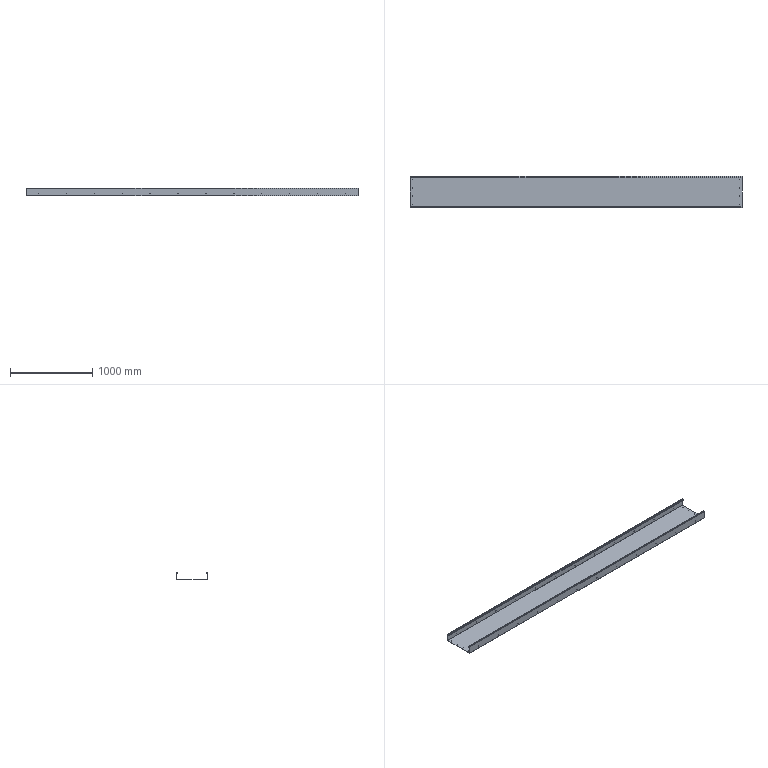Part | STEP file | TS-S80 | 1 solid | 118 faces | box 4045 x 380 x 97 mm | volume 5054054 mm3 | cylinder 76 | plane 42 | commonest cylinder face diameters 5.4 x64 0.4 x6 4.4 x6